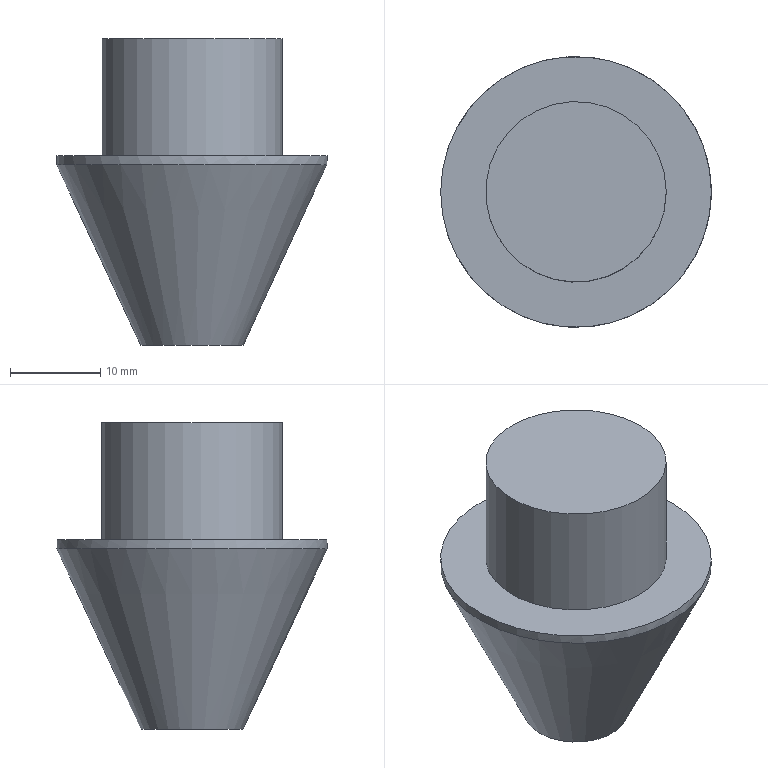Part | NX | features DATUM_CSYS 3, SKETCH 2, EXTRUDE 1, SWP104 1 | 1 solid | 6 faces | box 30 x 30 x 34 mm | volume 11960 mm3 | plane 3 | cylinder 2 | cone 1 | commonest cylinder face diameters 20 x1 30 x1
STEP:
#1=CARTESIAN_POINT('',(-15.,0.,20.));
#2=VERTEX_POINT('',#1);
#3=CARTESIAN_POINT('',(0.,0.,20.));
#4=DIRECTION('',(0.,0.,-1.));
#5=DIRECTION('',(-1.,0.,0.));
#6=AXIS2_PLACEMENT_3D('',#3,#4,#5);
#7=CIRCLE('',#6,15.);
#8=EDGE_CURVE('',#2,#2,#7,.T.);
#9=ORIENTED_EDGE('',*,*,#8,.F.);
#10=EDGE_LOOP('',(#9));
#11=FACE_BOUND('',#10,.T.);
#12=CARTESIAN_POINT('',(15.,0.,21.));
#13=VERTEX_POINT('',#12);
#14=CARTESIAN_POINT('',(0.,0.,21.));
#15=DIRECTION('',(0.,0.,1.));
#16=DIRECTION('',(1.,0.,0.));
#17=AXIS2_PLACEMENT_3D('',#14,#15,#16);
#18=CIRCLE('',#17,15.);
#19=EDGE_CURVE('',#13,#13,#18,.F.);
#20=ORIENTED_EDGE('',*,*,#19,.T.);
#21=EDGE_LOOP('',(#20));
#22=FACE_BOUND('',#21,.T.);
#23=CARTESIAN_POINT('',(0.,0.,0.));
#24=DIRECTION('',(0.,0.,-1.));
#25=DIRECTION('',(-1.,0.,0.));
#26=AXIS2_PLACEMENT_3D('',#23,#24,#25);
#27=CYLINDRICAL_SURFACE('',#26,15.);
#28=ADVANCED_FACE('',(#11,#22),#27,.T.);
#29=CARTESIAN_POINT('',(-5.674,0.,0.));
#30=VERTEX_POINT('',#29);
#31=CARTESIAN_POINT('',(0.,0.,0.));
#32=DIRECTION('',(0.,0.,-1.));
#33=DIRECTION('',(-1.,0.,0.));
#34=AXIS2_PLACEMENT_3D('',#31,#32,#33);
#35=CIRCLE('',#34,5.674);
#36=EDGE_CURVE('',#30,#30,#35,.T.);
#37=ORIENTED_EDGE('',*,*,#36,.T.);
#38=EDGE_LOOP('',(#37));
#39=FACE_BOUND('',#38,.T.);
#40=CARTESIAN_POINT('',(0.,0.,0.));
#41=DIRECTION('',(0.,0.,-1.));
#42=DIRECTION('',(-1.,0.,0.));
#43=AXIS2_PLACEMENT_3D('',#40,#41,#42);
#44=PLANE('',#43);
#45=ADVANCED_FACE('',(#39),#44,.T.);
#46=ORIENTED_EDGE('',*,*,#8,.T.);
#47=EDGE_LOOP('',(#46));
#48=FACE_BOUND('',#47,.T.);
#49=ORIENTED_EDGE('',*,*,#36,.F.);
#50=EDGE_LOOP('',(#49));
#51=FACE_BOUND('',#50,.T.);
#52=CARTESIAN_POINT('',(0.,0.,0.));
#53=DIRECTION('',(0.,0.,1.));
#54=DIRECTION('',(1.,0.,0.));
#55=AXIS2_PLACEMENT_3D('',#52,#53,#54);
#56=CONICAL_SURFACE('',#55,5.674,0.4363);
#57=ADVANCED_FACE('',(#48,#51),#56,.T.);
#58=CARTESIAN_POINT('',(10.,0.,21.));
#59=VERTEX_POINT('',#58);
#60=CARTESIAN_POINT('',(0.,0.,21.));
#61=DIRECTION('',(0.,0.,1.));
#62=DIRECTION('',(1.,0.,0.));
#63=AXIS2_PLACEMENT_3D('',#60,#61,#62);
#64=CIRCLE('',#63,10.);
#65=EDGE_CURVE('',#59,#59,#64,.F.);
#66=ORIENTED_EDGE('',*,*,#65,.F.);
#67=EDGE_LOOP('',(#66));
#68=FACE_BOUND('',#67,.T.);
#69=CARTESIAN_POINT('',(10.,0.,34.));
#70=VERTEX_POINT('',#69);
#71=CARTESIAN_POINT('',(0.,0.,34.));
#72=DIRECTION('',(0.,0.,1.));
#73=DIRECTION('',(1.,0.,0.));
#74=AXIS2_PLACEMENT_3D('',#71,#72,#73);
#75=CIRCLE('',#74,10.);
#76=EDGE_CURVE('',#70,#70,#75,.T.);
#77=ORIENTED_EDGE('',*,*,#76,.F.);
#78=EDGE_LOOP('',(#77));
#79=FACE_BOUND('',#78,.T.);
#80=CARTESIAN_POINT('',(0.,0.,21.));
#81=DIRECTION('',(0.,0.,1.));
#82=DIRECTION('',(1.,0.,0.));
#83=AXIS2_PLACEMENT_3D('',#80,#81,#82);
#84=CYLINDRICAL_SURFACE('',#83,10.);
#85=ADVANCED_FACE('',(#68,#79),#84,.T.);
#86=ORIENTED_EDGE('',*,*,#19,.F.);
#87=EDGE_LOOP('',(#86));
#88=FACE_BOUND('',#87,.T.);
#89=ORIENTED_EDGE('',*,*,#65,.T.);
#90=EDGE_LOOP('',(#89));
#91=FACE_BOUND('',#90,.T.);
#92=CARTESIAN_POINT('',(0.,0.,21.));
#93=DIRECTION('',(0.,0.,1.));
#94=DIRECTION('',(1.,0.,0.));
#95=AXIS2_PLACEMENT_3D('',#92,#93,#94);
#96=PLANE('',#95);
#97=ADVANCED_FACE('',(#88,#91),#96,.T.);
#98=ORIENTED_EDGE('',*,*,#76,.T.);
#99=EDGE_LOOP('',(#98));
#100=FACE_BOUND('',#99,.T.);
#101=CARTESIAN_POINT('',(15.,0.,34.));
#102=DIRECTION('',(0.,0.,1.));
#103=DIRECTION('',(1.,0.,0.));
#104=AXIS2_PLACEMENT_3D('',#101,#102,#103);
#105=PLANE('',#104);
#106=ADVANCED_FACE('',(#100),#105,.T.);
#107=CLOSED_SHELL('',(#28,#45,#57,#85,#97,#106));
#108=MANIFOLD_SOLID_BREP('',#107);
#109=(LENGTH_UNIT()NAMED_UNIT(*)SI_UNIT(.MILLI.,.METRE.));
#110=UNCERTAINTY_MEASURE_WITH_UNIT(LENGTH_MEASURE(0.00001),#109,'','');
#111=(NAMED_UNIT(*)PLANE_ANGLE_UNIT()SI_UNIT($,.RADIAN.));
#112=(NAMED_UNIT(*)SI_UNIT($,.STERADIAN.)SOLID_ANGLE_UNIT());
#113=(GEOMETRIC_REPRESENTATION_CONTEXT(3)GLOBAL_UNCERTAINTY_ASSIGNED_CONTEXT((#110))GLOBAL_UNIT_ASSIGNED_CONTEXT((#109,#111,#112))REPRESENTATION_CONTEXT('',''));
#114=ADVANCED_BREP_SHAPE_REPRESENTATION('',(#108),#113);